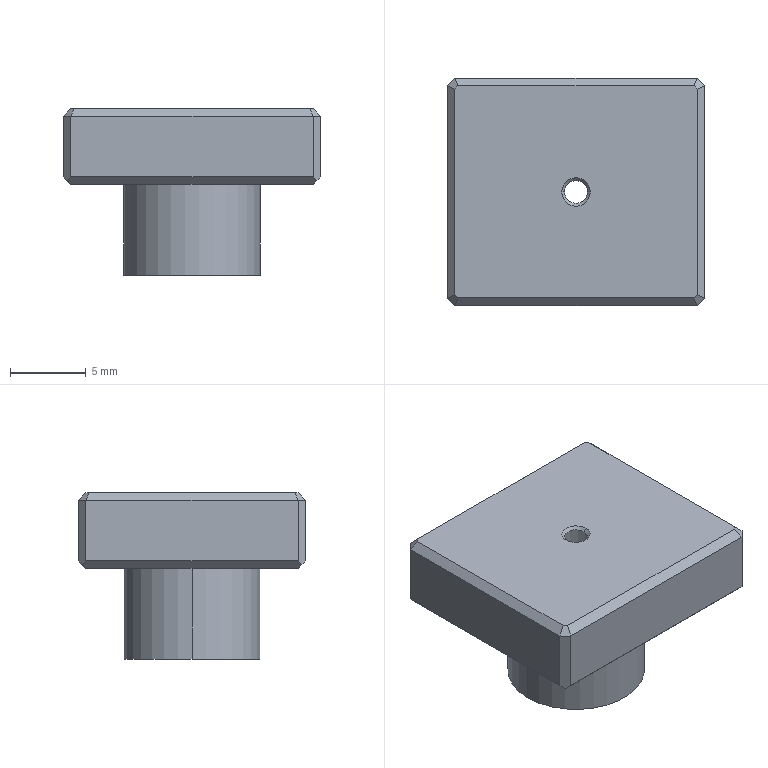Part | SolidWorks | features Chamfer 2, Extrusion 1, HoleWzd 1, ICE 1 | 1 solid | 31 faces | box 17 x 15 x 11 mm | volume 1494 mm3 | plane 23 | cone 4 | cylinder 4 | commonest cylinder face diameters 4.2 x2 9 x2
STEP:
#1=CARTESIAN_POINT('',(-0.7481,0.,10.812));
#2=VERTEX_POINT('',#1);
#3=CARTESIAN_POINT('',(0.7481,0.,10.812));
#4=VERTEX_POINT('',#3);
#5=CARTESIAN_POINT('',(0.,0.,10.812));
#6=DIRECTION('',(0.,0.,1.));
#7=DIRECTION('',(-1.,0.,0.));
#8=AXIS2_PLACEMENT_3D('',#5,#6,#7);
#9=CIRCLE('',#8,0.7481);
#10=EDGE_CURVE('',#2,#4,#9,.T.);
#11=ORIENTED_EDGE('',*,*,#10,.F.);
#12=CARTESIAN_POINT('',(-0.9357,0.,11.));
#13=VERTEX_POINT('',#12);
#14=CARTESIAN_POINT('',(-0.7481,0.,10.812));
#15=DIRECTION('',(-0.7071,0.,0.7071));
#16=VECTOR('',#15,1000.);
#17=LINE('',#14,#16);
#18=EDGE_CURVE('',#2,#13,#17,.T.);
#19=ORIENTED_EDGE('',*,*,#18,.T.);
#20=CARTESIAN_POINT('',(0.9357,0.,11.));
#21=VERTEX_POINT('',#20);
#22=CARTESIAN_POINT('',(0.,0.,11.));
#23=DIRECTION('',(0.,0.,-1.));
#24=DIRECTION('',(1.,0.,0.));
#25=AXIS2_PLACEMENT_3D('',#22,#23,#24);
#26=CIRCLE('',#25,0.9357);
#27=EDGE_CURVE('',#21,#13,#26,.T.);
#28=ORIENTED_EDGE('',*,*,#27,.F.);
#29=CARTESIAN_POINT('',(0.7481,0.,10.812));
#30=DIRECTION('',(0.7071,0.,0.7071));
#31=VECTOR('',#30,1000.);
#32=LINE('',#29,#31);
#33=EDGE_CURVE('',#4,#21,#32,.T.);
#34=ORIENTED_EDGE('',*,*,#33,.F.);
#35=EDGE_LOOP('',(#11,#19,#28,#34));
#36=FACE_OUTER_BOUND('',#35,.T.);
#37=CARTESIAN_POINT('',(0.,0.,10.812));
#38=DIRECTION('',(0.,0.,1.));
#39=DIRECTION('',(1.,0.,0.));
#40=AXIS2_PLACEMENT_3D('',#37,#38,#39);
#41=CONICAL_SURFACE('',#40,0.7481,0.7854);
#42=ADVANCED_FACE('',(#36),#41,.F.);
#43=CARTESIAN_POINT('',(2.1,0.,10.));
#44=VERTEX_POINT('',#43);
#45=CARTESIAN_POINT('',(-2.1,0.,10.));
#46=VERTEX_POINT('',#45);
#47=CARTESIAN_POINT('',(0.,0.,10.));
#48=DIRECTION('',(0.,0.,-1.));
#49=DIRECTION('',(-1.,0.,0.));
#50=AXIS2_PLACEMENT_3D('',#47,#48,#49);
#51=CIRCLE('',#50,2.1);
#52=EDGE_CURVE('',#44,#46,#51,.T.);
#53=ORIENTED_EDGE('',*,*,#52,.F.);
#54=CARTESIAN_POINT('',(2.1,0.,0.));
#55=VERTEX_POINT('',#54);
#56=CARTESIAN_POINT('',(2.1,0.,0.));
#57=DIRECTION('',(0.,0.,-1.));
#58=VECTOR('',#57,1000.);
#59=LINE('',#56,#58);
#60=EDGE_CURVE('',#44,#55,#59,.T.);
#61=ORIENTED_EDGE('',*,*,#60,.T.);
#62=CARTESIAN_POINT('',(-2.1,0.,0.));
#63=VERTEX_POINT('',#62);
#64=CARTESIAN_POINT('',(0.,0.,0.));
#65=DIRECTION('',(0.,0.,-1.));
#66=DIRECTION('',(-1.,0.,0.));
#67=AXIS2_PLACEMENT_3D('',#64,#65,#66);
#68=CIRCLE('',#67,2.1);
#69=EDGE_CURVE('',#55,#63,#68,.T.);
#70=ORIENTED_EDGE('',*,*,#69,.T.);
#71=CARTESIAN_POINT('',(-2.1,0.,0.));
#72=DIRECTION('',(0.,0.,-1.));
#73=VECTOR('',#72,1000.);
#74=LINE('',#71,#73);
#75=EDGE_CURVE('',#46,#63,#74,.T.);
#76=ORIENTED_EDGE('',*,*,#75,.F.);
#77=EDGE_LOOP('',(#53,#61,#70,#76));
#78=FACE_OUTER_BOUND('',#77,.T.);
#79=CARTESIAN_POINT('',(0.,0.,0.));
#80=DIRECTION('',(0.,0.,-1.));
#81=DIRECTION('',(-1.,0.,0.));
#82=AXIS2_PLACEMENT_3D('',#79,#80,#81);
#83=CYLINDRICAL_SURFACE('',#82,2.1);
#84=ADVANCED_FACE('',(#78),#83,.F.);
#85=ORIENTED_EDGE('',*,*,#10,.T.);
#86=CARTESIAN_POINT('',(2.1,0.,10.));
#87=DIRECTION('',(0.8572,0.,-0.515));
#88=VECTOR('',#87,1000.);
#89=LINE('',#86,#88);
#90=EDGE_CURVE('',#4,#44,#89,.T.);
#91=ORIENTED_EDGE('',*,*,#90,.T.);
#92=ORIENTED_EDGE('',*,*,#52,.T.);
#93=CARTESIAN_POINT('',(-2.1,0.,10.));
#94=DIRECTION('',(-0.8572,0.,-0.515));
#95=VECTOR('',#94,1000.);
#96=LINE('',#93,#95);
#97=EDGE_CURVE('',#2,#46,#96,.T.);
#98=ORIENTED_EDGE('',*,*,#97,.F.);
#99=EDGE_LOOP('',(#85,#91,#92,#98));
#100=FACE_OUTER_BOUND('',#99,.T.);
#101=CARTESIAN_POINT('',(0.,0.,10.));
#102=DIRECTION('',(0.,0.,-1.));
#103=DIRECTION('',(-1.,0.,0.));
#104=AXIS2_PLACEMENT_3D('',#101,#102,#103);
#105=CONICAL_SURFACE('',#104,2.1,1.03);
#106=ADVANCED_FACE('',(#100),#105,.F.);
#107=CARTESIAN_POINT('',(4.5,0.,6.));
#108=VERTEX_POINT('',#107);
#109=CARTESIAN_POINT('',(-4.5,0.,6.));
#110=VERTEX_POINT('',#109);
#111=CARTESIAN_POINT('',(0.,0.,6.));
#112=DIRECTION('',(0.,0.,1.));
#113=DIRECTION('',(1.,0.,0.));
#114=AXIS2_PLACEMENT_3D('',#111,#112,#113);
#115=CIRCLE('',#114,4.5);
#116=EDGE_CURVE('',#108,#110,#115,.T.);
#117=ORIENTED_EDGE('',*,*,#116,.F.);
#118=CARTESIAN_POINT('',(4.5,0.,0.));
#119=VERTEX_POINT('',#118);
#120=CARTESIAN_POINT('',(4.5,0.,6.));
#121=DIRECTION('',(0.,0.,-1.));
#122=VECTOR('',#121,1000.);
#123=LINE('',#120,#122);
#124=EDGE_CURVE('',#108,#119,#123,.T.);
#125=ORIENTED_EDGE('',*,*,#124,.T.);
#126=CARTESIAN_POINT('',(-4.5,0.,0.));
#127=VERTEX_POINT('',#126);
#128=CARTESIAN_POINT('',(0.,0.,0.));
#129=DIRECTION('',(0.,0.,1.));
#130=DIRECTION('',(1.,0.,0.));
#131=AXIS2_PLACEMENT_3D('',#128,#129,#130);
#132=CIRCLE('',#131,4.5);
#133=EDGE_CURVE('',#119,#127,#132,.T.);
#134=ORIENTED_EDGE('',*,*,#133,.T.);
#135=CARTESIAN_POINT('',(-4.5,0.,6.));
#136=DIRECTION('',(0.,0.,-1.));
#137=VECTOR('',#136,1000.);
#138=LINE('',#135,#137);
#139=EDGE_CURVE('',#110,#127,#138,.T.);
#140=ORIENTED_EDGE('',*,*,#139,.F.);
#141=EDGE_LOOP('',(#117,#125,#134,#140));
#142=FACE_OUTER_BOUND('',#141,.T.);
#143=CARTESIAN_POINT('',(0.,0.,6.));
#144=DIRECTION('',(0.,0.,-1.));
#145=DIRECTION('',(-1.,0.,0.));
#146=AXIS2_PLACEMENT_3D('',#143,#144,#145);
#147=CYLINDRICAL_SURFACE('',#146,4.5);
#148=ADVANCED_FACE('',(#142),#147,.T.);
#149=ORIENTED_EDGE('',*,*,#124,.F.);
#150=CARTESIAN_POINT('',(0.,0.,6.));
#151=DIRECTION('',(0.,0.,1.));
#152=DIRECTION('',(1.,0.,0.));
#153=AXIS2_PLACEMENT_3D('',#150,#151,#152);
#154=CIRCLE('',#153,4.5);
#155=EDGE_CURVE('',#110,#108,#154,.T.);
#156=ORIENTED_EDGE('',*,*,#155,.F.);
#157=ORIENTED_EDGE('',*,*,#139,.T.);
#158=CARTESIAN_POINT('',(0.,0.,0.));
#159=DIRECTION('',(0.,0.,1.));
#160=DIRECTION('',(1.,0.,0.));
#161=AXIS2_PLACEMENT_3D('',#158,#159,#160);
#162=CIRCLE('',#161,4.5);
#163=EDGE_CURVE('',#127,#119,#162,.T.);
#164=ORIENTED_EDGE('',*,*,#163,.T.);
#165=EDGE_LOOP('',(#149,#156,#157,#164));
#166=FACE_OUTER_BOUND('',#165,.T.);
#167=CARTESIAN_POINT('',(0.,0.,6.));
#168=DIRECTION('',(0.,0.,-1.));
#169=DIRECTION('',(-1.,0.,0.));
#170=AXIS2_PLACEMENT_3D('',#167,#168,#169);
#171=CYLINDRICAL_SURFACE('',#170,4.5);
#172=ADVANCED_FACE('',(#166),#171,.T.);
#173=CARTESIAN_POINT('',(0.,0.,0.));
#174=DIRECTION('',(0.,0.,-1.));
#175=DIRECTION('',(-1.,0.,0.));
#176=AXIS2_PLACEMENT_3D('',#173,#174,#175);
#177=CIRCLE('',#176,2.1);
#178=EDGE_CURVE('',#63,#55,#177,.T.);
#179=ORIENTED_EDGE('',*,*,#178,.F.);
#180=ORIENTED_EDGE('',*,*,#69,.F.);
#181=EDGE_LOOP('',(#179,#180));
#182=FACE_BOUND('',#181,.T.);
#183=ORIENTED_EDGE('',*,*,#163,.F.);
#184=ORIENTED_EDGE('',*,*,#133,.F.);
#185=EDGE_LOOP('',(#183,#184));
#186=FACE_OUTER_BOUND('',#185,.T.);
#187=CARTESIAN_POINT('',(0.,0.,0.));
#188=DIRECTION('',(0.,0.,1.));
#189=DIRECTION('',(1.,0.,0.));
#190=AXIS2_PLACEMENT_3D('',#187,#188,#189);
#191=PLANE('',#190);
#192=ADVANCED_FACE('',(#182,#186),#191,.F.);
#193=CARTESIAN_POINT('',(8.5,7.,6.5));
#194=VERTEX_POINT('',#193);
#195=CARTESIAN_POINT('',(8.5,7.,10.5));
#196=VERTEX_POINT('',#195);
#197=CARTESIAN_POINT('',(8.5,7.,11.));
#198=DIRECTION('',(0.,0.,1.));
#199=VECTOR('',#198,1000.);
#200=LINE('',#197,#199);
#201=EDGE_CURVE('',#194,#196,#200,.T.);
#202=ORIENTED_EDGE('',*,*,#201,.T.);
#203=CARTESIAN_POINT('',(8.5,-7.,10.5));
#204=VERTEX_POINT('',#203);
#205=CARTESIAN_POINT('',(8.5,-7.,10.5));
#206=DIRECTION('',(0.,-1.,0.));
#207=VECTOR('',#206,1000.);
#208=LINE('',#205,#207);
#209=EDGE_CURVE('',#196,#204,#208,.T.);
#210=ORIENTED_EDGE('',*,*,#209,.T.);
#211=CARTESIAN_POINT('',(8.5,-7.,6.5));
#212=VERTEX_POINT('',#211);
#213=CARTESIAN_POINT('',(8.5,-7.,11.));
#214=DIRECTION('',(0.,0.,-1.));
#215=VECTOR('',#214,1000.);
#216=LINE('',#213,#215);
#217=EDGE_CURVE('',#204,#212,#216,.T.);
#218=ORIENTED_EDGE('',*,*,#217,.T.);
#219=CARTESIAN_POINT('',(8.5,7.5,6.5));
#220=DIRECTION('',(0.,1.,0.));
#221=VECTOR('',#220,1000.);
#222=LINE('',#219,#221);
#223=EDGE_CURVE('',#212,#194,#222,.T.);
#224=ORIENTED_EDGE('',*,*,#223,.T.);
#225=EDGE_LOOP('',(#202,#210,#218,#224));
#226=FACE_OUTER_BOUND('',#225,.T.);
#227=CARTESIAN_POINT('',(8.5,7.5,11.));
#228=DIRECTION('',(-1.,0.,0.));
#229=DIRECTION('',(0.,-1.,0.));
#230=AXIS2_PLACEMENT_3D('',#227,#228,#229);
#231=PLANE('',#230);
#232=ADVANCED_FACE('',(#226),#231,.F.);
#233=CARTESIAN_POINT('',(-8.,7.5,6.5));
#234=VERTEX_POINT('',#233);
#235=CARTESIAN_POINT('',(-8.,7.5,10.5));
#236=VERTEX_POINT('',#235);
#237=CARTESIAN_POINT('',(-8.,7.5,11.));
#238=DIRECTION('',(0.,0.,1.));
#239=VECTOR('',#238,1000.);
#240=LINE('',#237,#239);
#241=EDGE_CURVE('',#234,#236,#240,.T.);
#242=ORIENTED_EDGE('',*,*,#241,.T.);
#243=CARTESIAN_POINT('',(8.,7.5,10.5));
#244=VERTEX_POINT('',#243);
#245=CARTESIAN_POINT('',(8.,7.5,10.5));
#246=DIRECTION('',(1.,0.,0.));
#247=VECTOR('',#246,1000.);
#248=LINE('',#245,#247);
#249=EDGE_CURVE('',#236,#244,#248,.T.);
#250=ORIENTED_EDGE('',*,*,#249,.T.);
#251=CARTESIAN_POINT('',(8.,7.5,6.5));
#252=VERTEX_POINT('',#251);
#253=CARTESIAN_POINT('',(8.,7.5,11.));
#254=DIRECTION('',(0.,0.,-1.));
#255=VECTOR('',#254,1000.);
#256=LINE('',#253,#255);
#257=EDGE_CURVE('',#244,#252,#256,.T.);
#258=ORIENTED_EDGE('',*,*,#257,.T.);
#259=CARTESIAN_POINT('',(-8.5,7.5,6.5));
#260=DIRECTION('',(-1.,0.,0.));
#261=VECTOR('',#260,1000.);
#262=LINE('',#259,#261);
#263=EDGE_CURVE('',#252,#234,#262,.T.);
#264=ORIENTED_EDGE('',*,*,#263,.T.);
#265=EDGE_LOOP('',(#242,#250,#258,#264));
#266=FACE_OUTER_BOUND('',#265,.T.);
#267=CARTESIAN_POINT('',(-8.5,7.5,11.));
#268=DIRECTION('',(0.,-1.,0.));
#269=DIRECTION('',(0.,0.,-1.));
#270=AXIS2_PLACEMENT_3D('',#267,#268,#269);
#271=PLANE('',#270);
#272=ADVANCED_FACE('',(#266),#271,.F.);
#273=CARTESIAN_POINT('',(-8.5,-7.,6.5));
#274=VERTEX_POINT('',#273);
#275=CARTESIAN_POINT('',(-8.5,-7.,10.5));
#276=VERTEX_POINT('',#275);
#277=CARTESIAN_POINT('',(-8.5,-7.,11.));
#278=DIRECTION('',(0.,0.,1.));
#279=VECTOR('',#278,1000.);
#280=LINE('',#277,#279);
#281=EDGE_CURVE('',#274,#276,#280,.T.);
#282=ORIENTED_EDGE('',*,*,#281,.T.);
#283=CARTESIAN_POINT('',(-8.5,7.,10.5));
#284=VERTEX_POINT('',#283);
#285=CARTESIAN_POINT('',(-8.5,7.,10.5));
#286=DIRECTION('',(0.,1.,0.));
#287=VECTOR('',#286,1000.);
#288=LINE('',#285,#287);
#289=EDGE_CURVE('',#276,#284,#288,.T.);
#290=ORIENTED_EDGE('',*,*,#289,.T.);
#291=CARTESIAN_POINT('',(-8.5,7.,6.5));
#292=VERTEX_POINT('',#291);
#293=CARTESIAN_POINT('',(-8.5,7.,11.));
#294=DIRECTION('',(0.,0.,-1.));
#295=VECTOR('',#294,1000.);
#296=LINE('',#293,#295);
#297=EDGE_CURVE('',#284,#292,#296,.T.);
#298=ORIENTED_EDGE('',*,*,#297,.T.);
#299=CARTESIAN_POINT('',(-8.5,7.5,6.5));
#300=DIRECTION('',(0.,-1.,0.));
#301=VECTOR('',#300,1000.);
#302=LINE('',#299,#301);
#303=EDGE_CURVE('',#292,#274,#302,.T.);
#304=ORIENTED_EDGE('',*,*,#303,.T.);
#305=EDGE_LOOP('',(#282,#290,#298,#304));
#306=FACE_OUTER_BOUND('',#305,.T.);
#307=CARTESIAN_POINT('',(-8.5,7.5,11.));
#308=DIRECTION('',(1.,0.,0.));
#309=DIRECTION('',(0.,1.,0.));
#310=AXIS2_PLACEMENT_3D('',#307,#308,#309);
#311=PLANE('',#310);
#312=ADVANCED_FACE('',(#306),#311,.F.);
#313=CARTESIAN_POINT('',(8.,-7.5,6.5));
#314=VERTEX_POINT('',#313);
#315=CARTESIAN_POINT('',(8.,-7.5,10.5));
#316=VERTEX_POINT('',#315);
#317=CARTESIAN_POINT('',(8.,-7.5,11.));
#318=DIRECTION('',(0.,0.,1.));
#319=VECTOR('',#318,1000.);
#320=LINE('',#317,#319);
#321=EDGE_CURVE('',#314,#316,#320,.T.);
#322=ORIENTED_EDGE('',*,*,#321,.T.);
#323=CARTESIAN_POINT('',(-8.,-7.5,10.5));
#324=VERTEX_POINT('',#323);
#325=CARTESIAN_POINT('',(-8.,-7.5,10.5));
#326=DIRECTION('',(-1.,0.,0.));
#327=VECTOR('',#326,1000.);
#328=LINE('',#325,#327);
#329=EDGE_CURVE('',#316,#324,#328,.T.);
#330=ORIENTED_EDGE('',*,*,#329,.T.);
#331=CARTESIAN_POINT('',(-8.,-7.5,6.5));
#332=VERTEX_POINT('',#331);
#333=CARTESIAN_POINT('',(-8.,-7.5,11.));
#334=DIRECTION('',(0.,0.,-1.));
#335=VECTOR('',#334,1000.);
#336=LINE('',#333,#335);
#337=EDGE_CURVE('',#324,#332,#336,.T.);
#338=ORIENTED_EDGE('',*,*,#337,.T.);
#339=CARTESIAN_POINT('',(-8.5,-7.5,6.5));
#340=DIRECTION('',(1.,0.,0.));
#341=VECTOR('',#340,1000.);
#342=LINE('',#339,#341);
#343=EDGE_CURVE('',#332,#314,#342,.T.);
#344=ORIENTED_EDGE('',*,*,#343,.T.);
#345=EDGE_LOOP('',(#322,#330,#338,#344));
#346=FACE_OUTER_BOUND('',#345,.T.);
#347=CARTESIAN_POINT('',(-8.5,-7.5,11.));
#348=DIRECTION('',(0.,1.,0.));
#349=DIRECTION('',(0.,0.,1.));
#350=AXIS2_PLACEMENT_3D('',#347,#348,#349);
#351=PLANE('',#350);
#352=ADVANCED_FACE('',(#346),#351,.F.);
#353=CARTESIAN_POINT('',(-8.,6.793,11.));
#354=VERTEX_POINT('',#353);
#355=CARTESIAN_POINT('',(-8.,-6.793,11.));
#356=VERTEX_POINT('',#355);
#357=CARTESIAN_POINT('',(-8.,-7.,11.));
#358=DIRECTION('',(0.,-1.,0.));
#359=VECTOR('',#358,1000.);
#360=LINE('',#357,#359);
#361=EDGE_CURVE('',#354,#356,#360,.T.);
#362=ORIENTED_EDGE('',*,*,#361,.T.);
#363=CARTESIAN_POINT('',(-7.793,-7.,11.));
#364=VERTEX_POINT('',#363);
#365=CARTESIAN_POINT('',(-7.396,-7.396,11.));
#366=DIRECTION('',(0.7071,-0.7071,0.));
#367=VECTOR('',#366,1000.);
#368=LINE('',#365,#367);
#369=EDGE_CURVE('',#356,#364,#368,.T.);
#370=ORIENTED_EDGE('',*,*,#369,.T.);
#371=CARTESIAN_POINT('',(7.793,-7.,11.));
#372=VERTEX_POINT('',#371);
#373=CARTESIAN_POINT('',(8.,-7.,11.));
#374=DIRECTION('',(1.,0.,0.));
#375=VECTOR('',#374,1000.);
#376=LINE('',#373,#375);
#377=EDGE_CURVE('',#364,#372,#376,.T.);
#378=ORIENTED_EDGE('',*,*,#377,.T.);
#379=CARTESIAN_POINT('',(8.,-6.793,11.));
#380=VERTEX_POINT('',#379);
#381=CARTESIAN_POINT('',(7.396,-7.396,11.));
#382=DIRECTION('',(0.7071,0.7071,0.));
#383=VECTOR('',#382,1000.);
#384=LINE('',#381,#383);
#385=EDGE_CURVE('',#372,#380,#384,.T.);
#386=ORIENTED_EDGE('',*,*,#385,.T.);
#387=CARTESIAN_POINT('',(8.,6.793,11.));
#388=VERTEX_POINT('',#387);
#389=CARTESIAN_POINT('',(8.,7.,11.));
#390=DIRECTION('',(0.,1.,0.));
#391=VECTOR('',#390,1000.);
#392=LINE('',#389,#391);
#393=EDGE_CURVE('',#380,#388,#392,.T.);
#394=ORIENTED_EDGE('',*,*,#393,.T.);
#395=CARTESIAN_POINT('',(7.793,7.,11.));
#396=VERTEX_POINT('',#395);
#397=CARTESIAN_POINT('',(7.396,7.396,11.));
#398=DIRECTION('',(-0.7071,0.7071,0.));
#399=VECTOR('',#398,1000.);
#400=LINE('',#397,#399);
#401=EDGE_CURVE('',#388,#396,#400,.T.);
#402=ORIENTED_EDGE('',*,*,#401,.T.);
#403=CARTESIAN_POINT('',(-7.793,7.,11.));
#404=VERTEX_POINT('',#403);
#405=CARTESIAN_POINT('',(-8.,7.,11.));
#406=DIRECTION('',(-1.,0.,0.));
#407=VECTOR('',#406,1000.);
#408=LINE('',#405,#407);
#409=EDGE_CURVE('',#396,#404,#408,.T.);
#410=ORIENTED_EDGE('',*,*,#409,.T.);
#411=CARTESIAN_POINT('',(-7.396,7.396,11.));
#412=DIRECTION('',(-0.7071,-0.7071,0.));
#413=VECTOR('',#412,1000.);
#414=LINE('',#411,#413);
#415=EDGE_CURVE('',#404,#354,#414,.T.);
#416=ORIENTED_EDGE('',*,*,#415,.T.);
#417=EDGE_LOOP('',(#362,#370,#378,#386,#394,#402,#410,#416));
#418=FACE_OUTER_BOUND('',#417,.T.);
#419=ORIENTED_EDGE('',*,*,#27,.T.);
#420=CARTESIAN_POINT('',(0.,0.,11.));
#421=DIRECTION('',(0.,0.,-1.));
#422=DIRECTION('',(1.,0.,0.));
#423=AXIS2_PLACEMENT_3D('',#420,#421,#422);
#424=CIRCLE('',#423,0.9357);
#425=EDGE_CURVE('',#13,#21,#424,.T.);
#426=ORIENTED_EDGE('',*,*,#425,.T.);
#427=EDGE_LOOP('',(#419,#426));
#428=FACE_BOUND('',#427,.T.);
#429=CARTESIAN_POINT('',(0.,0.,11.));
#430=DIRECTION('',(0.,0.,1.));
#431=DIRECTION('',(1.,0.,0.));
#432=AXIS2_PLACEMENT_3D('',#429,#430,#431);
#433=PLANE('',#432);
#434=ADVANCED_FACE('',(#418,#428),#433,.T.);
#435=CARTESIAN_POINT('',(-8.,-7.,6.));
#436=VERTEX_POINT('',#435);
#437=CARTESIAN_POINT('',(-8.,7.,6.));
#438=VERTEX_POINT('',#437);
#439=CARTESIAN_POINT('',(-8.,0.,6.));
#440=DIRECTION('',(0.,1.,0.));
#441=VECTOR('',#440,1000.);
#442=LINE('',#439,#441);
#443=EDGE_CURVE('',#436,#438,#442,.T.);
#444=ORIENTED_EDGE('',*,*,#443,.T.);
#445=CARTESIAN_POINT('',(8.,7.,6.));
#446=VERTEX_POINT('',#445);
#447=CARTESIAN_POINT('',(0.,7.,6.));
#448=DIRECTION('',(1.,0.,0.));
#449=VECTOR('',#448,1000.);
#450=LINE('',#447,#449);
#451=EDGE_CURVE('',#438,#446,#450,.T.);
#452=ORIENTED_EDGE('',*,*,#451,.T.);
#453=CARTESIAN_POINT('',(8.,-7.,6.));
#454=VERTEX_POINT('',#453);
#455=CARTESIAN_POINT('',(8.,0.,6.));
#456=DIRECTION('',(0.,-1.,0.));
#457=VECTOR('',#456,1000.);
#458=LINE('',#455,#457);
#459=EDGE_CURVE('',#446,#454,#458,.T.);
#460=ORIENTED_EDGE('',*,*,#459,.T.);
#461=CARTESIAN_POINT('',(0.,-7.,6.));
#462=DIRECTION('',(-1.,0.,0.));
#463=VECTOR('',#462,1000.);
#464=LINE('',#461,#463);
#465=EDGE_CURVE('',#454,#436,#464,.T.);
#466=ORIENTED_EDGE('',*,*,#465,.T.);
#467=EDGE_LOOP('',(#444,#452,#460,#466));
#468=FACE_OUTER_BOUND('',#467,.T.);
#469=ORIENTED_EDGE('',*,*,#155,.T.);
#470=ORIENTED_EDGE('',*,*,#116,.T.);
#471=EDGE_LOOP('',(#469,#470));
#472=FACE_BOUND('',#471,.T.);
#473=CARTESIAN_POINT('',(0.,0.,6.));
#474=DIRECTION('',(0.,0.,1.));
#475=DIRECTION('',(1.,0.,0.));
#476=AXIS2_PLACEMENT_3D('',#473,#474,#475);
#477=PLANE('',#476);
#478=ADVANCED_FACE('',(#468,#472),#477,.F.);
#479=ORIENTED_EDGE('',*,*,#90,.F.);
#480=CARTESIAN_POINT('',(0.,0.,10.812));
#481=DIRECTION('',(0.,0.,1.));
#482=DIRECTION('',(-1.,0.,0.));
#483=AXIS2_PLACEMENT_3D('',#480,#481,#482);
#484=CIRCLE('',#483,0.7481);
#485=EDGE_CURVE('',#4,#2,#484,.T.);
#486=ORIENTED_EDGE('',*,*,#485,.T.);
#487=ORIENTED_EDGE('',*,*,#97,.T.);
#488=CARTESIAN_POINT('',(0.,0.,10.));
#489=DIRECTION('',(0.,0.,-1.));
#490=DIRECTION('',(-1.,0.,0.));
#491=AXIS2_PLACEMENT_3D('',#488,#489,#490);
#492=CIRCLE('',#491,2.1);
#493=EDGE_CURVE('',#46,#44,#492,.T.);
#494=ORIENTED_EDGE('',*,*,#493,.T.);
#495=EDGE_LOOP('',(#479,#486,#487,#494));
#496=FACE_OUTER_BOUND('',#495,.T.);
#497=CARTESIAN_POINT('',(0.,0.,10.));
#498=DIRECTION('',(0.,0.,-1.));
#499=DIRECTION('',(-1.,0.,0.));
#500=AXIS2_PLACEMENT_3D('',#497,#498,#499);
#501=CONICAL_SURFACE('',#500,2.1,1.03);
#502=ADVANCED_FACE('',(#496),#501,.F.);
#503=ORIENTED_EDGE('',*,*,#60,.F.);
#504=ORIENTED_EDGE('',*,*,#493,.F.);
#505=ORIENTED_EDGE('',*,*,#75,.T.);
#506=ORIENTED_EDGE('',*,*,#178,.T.);
#507=EDGE_LOOP('',(#503,#504,#505,#506));
#508=FACE_OUTER_BOUND('',#507,.T.);
#509=CARTESIAN_POINT('',(0.,0.,0.));
#510=DIRECTION('',(0.,0.,-1.));
#511=DIRECTION('',(-1.,0.,0.));
#512=AXIS2_PLACEMENT_3D('',#509,#510,#511);
#513=CYLINDRICAL_SURFACE('',#512,2.1);
#514=ADVANCED_FACE('',(#508),#513,.F.);
#515=ORIENTED_EDGE('',*,*,#217,.F.);
#516=CARTESIAN_POINT('',(8.5,-7.,10.5));
#517=DIRECTION('',(-0.7071,-0.7071,0.));
#518=VECTOR('',#517,1000.);
#519=LINE('',#516,#518);
#520=EDGE_CURVE('',#204,#316,#519,.T.);
#521=ORIENTED_EDGE('',*,*,#520,.T.);
#522=ORIENTED_EDGE('',*,*,#321,.F.);
#523=CARTESIAN_POINT('',(8.25,-7.25,6.25));
#524=VERTEX_POINT('',#523);
#525=CARTESIAN_POINT('',(6.833,-8.667,7.667));
#526=DIRECTION('',(0.5774,0.5774,-0.5774));
#527=VECTOR('',#526,1000.);
#528=LINE('',#525,#527);
#529=EDGE_CURVE('',#314,#524,#528,.T.);
#530=ORIENTED_EDGE('',*,*,#529,.T.);
#531=CARTESIAN_POINT('',(10.,-5.5,8.));
#532=DIRECTION('',(0.5774,0.5774,0.5774));
#533=VECTOR('',#532,1000.);
#534=LINE('',#531,#533);
#535=EDGE_CURVE('',#524,#212,#534,.T.);
#536=ORIENTED_EDGE('',*,*,#535,.T.);
#537=EDGE_LOOP('',(#515,#521,#522,#530,#536));
#538=FACE_OUTER_BOUND('',#537,.T.);
#539=CARTESIAN_POINT('',(8.5,-7.,11.));
#540=DIRECTION('',(-0.7071,0.7071,0.));
#541=DIRECTION('',(0.,0.,-1.));
#542=AXIS2_PLACEMENT_3D('',#539,#540,#541);
#543=PLANE('',#542);
#544=ADVANCED_FACE('',(#538),#543,.F.);
#545=ORIENTED_EDGE('',*,*,#257,.F.);
#546=CARTESIAN_POINT('',(8.,7.5,10.5));
#547=DIRECTION('',(0.7071,-0.7071,0.));
#548=VECTOR('',#547,1000.);
#549=LINE('',#546,#548);
#550=EDGE_CURVE('',#244,#196,#549,.T.);
#551=ORIENTED_EDGE('',*,*,#550,.T.);
#552=ORIENTED_EDGE('',*,*,#201,.F.);
#553=CARTESIAN_POINT('',(8.25,7.25,6.25));
#554=VERTEX_POINT('',#553);
#555=CARTESIAN_POINT('',(9.667,5.833,7.667));
#556=DIRECTION('',(-0.5774,0.5774,-0.5774));
#557=VECTOR('',#556,1000.);
#558=LINE('',#555,#557);
#559=EDGE_CURVE('',#194,#554,#558,.T.);
#560=ORIENTED_EDGE('',*,*,#559,.T.);
#561=CARTESIAN_POINT('',(6.5,9.,8.));
#562=DIRECTION('',(-0.5774,0.5774,0.5774));
#563=VECTOR('',#562,1000.);
#564=LINE('',#561,#563);
#565=EDGE_CURVE('',#554,#252,#564,.T.);
#566=ORIENTED_EDGE('',*,*,#565,.T.);
#567=EDGE_LOOP('',(#545,#551,#552,#560,#566));
#568=FACE_OUTER_BOUND('',#567,.T.);
#569=CARTESIAN_POINT('',(8.,7.5,11.));
#570=DIRECTION('',(-0.7071,-0.7071,0.));
#571=DIRECTION('',(0.,0.,-1.));
#572=AXIS2_PLACEMENT_3D('',#569,#570,#571);
#573=PLANE('',#572);
#574=ADVANCED_FACE('',(#568),#573,.F.);
#575=ORIENTED_EDGE('',*,*,#337,.F.);
#576=CARTESIAN_POINT('',(-8.,-7.5,10.5));
#577=DIRECTION('',(-0.7071,0.7071,0.));
#578=VECTOR('',#577,1000.);
#579=LINE('',#576,#578);
#580=EDGE_CURVE('',#324,#276,#579,.T.);
#581=ORIENTED_EDGE('',*,*,#580,.T.);
#582=ORIENTED_EDGE('',*,*,#281,.F.);
#583=CARTESIAN_POINT('',(-8.25,-7.25,6.25));
#584=VERTEX_POINT('',#583);
#585=CARTESIAN_POINT('',(-9.667,-5.833,7.667));
#586=DIRECTION('',(0.5774,-0.5774,-0.5774));
#587=VECTOR('',#586,1000.);
#588=LINE('',#585,#587);
#589=EDGE_CURVE('',#274,#584,#588,.T.);
#590=ORIENTED_EDGE('',*,*,#589,.T.);
#591=CARTESIAN_POINT('',(-6.5,-9.,8.));
#592=DIRECTION('',(0.5774,-0.5774,0.5774));
#593=VECTOR('',#592,1000.);
#594=LINE('',#591,#593);
#595=EDGE_CURVE('',#584,#332,#594,.T.);
#596=ORIENTED_EDGE('',*,*,#595,.T.);
#597=EDGE_LOOP('',(#575,#581,#582,#590,#596));
#598=FACE_OUTER_BOUND('',#597,.T.);
#599=CARTESIAN_POINT('',(-8.,-7.5,11.));
#600=DIRECTION('',(0.7071,0.7071,0.));
#601=DIRECTION('',(0.,0.,-1.));
#602=AXIS2_PLACEMENT_3D('',#599,#600,#601);
#603=PLANE('',#602);
#604=ADVANCED_FACE('',(#598),#603,.F.);
#605=ORIENTED_EDGE('',*,*,#297,.F.);
#606=CARTESIAN_POINT('',(-8.5,7.,10.5));
#607=DIRECTION('',(0.7071,0.7071,0.));
#608=VECTOR('',#607,1000.);
#609=LINE('',#606,#608);
#610=EDGE_CURVE('',#284,#236,#609,.T.);
#611=ORIENTED_EDGE('',*,*,#610,.T.);
#612=ORIENTED_EDGE('',*,*,#241,.F.);
#613=CARTESIAN_POINT('',(-8.25,7.25,6.25));
#614=VERTEX_POINT('',#613);
#615=CARTESIAN_POINT('',(-6.833,8.667,7.667));
#616=DIRECTION('',(-0.5774,-0.5774,-0.5774));
#617=VECTOR('',#616,1000.);
#618=LINE('',#615,#617);
#619=EDGE_CURVE('',#234,#614,#618,.T.);
#620=ORIENTED_EDGE('',*,*,#619,.T.);
#621=CARTESIAN_POINT('',(-10.,5.5,8.));
#622=DIRECTION('',(-0.5774,-0.5774,0.5774));
#623=VECTOR('',#622,1000.);
#624=LINE('',#621,#623);
#625=EDGE_CURVE('',#614,#292,#624,.T.);
#626=ORIENTED_EDGE('',*,*,#625,.T.);
#627=EDGE_LOOP('',(#605,#611,#612,#620,#626));
#628=FACE_OUTER_BOUND('',#627,.T.);
#629=CARTESIAN_POINT('',(-8.5,7.,11.));
#630=DIRECTION('',(0.7071,-0.7071,0.));
#631=DIRECTION('',(0.,0.,-1.));
#632=AXIS2_PLACEMENT_3D('',#629,#630,#631);
#633=PLANE('',#632);
#634=ADVANCED_FACE('',(#628),#633,.F.);
#635=CARTESIAN_POINT('',(6.704,6.256,12.296));
#636=DIRECTION('',(-0.6786,-0.2811,0.6786));
#637=VECTOR('',#636,1000.);
#638=LINE('',#635,#637);
#639=EDGE_CURVE('',#196,#388,#638,.T.);
#640=ORIENTED_EDGE('',*,*,#639,.F.);
#641=ORIENTED_EDGE('',*,*,#550,.F.);
#642=CARTESIAN_POINT('',(7.837,7.107,10.893));
#643=DIRECTION('',(0.2811,0.6786,-0.6786));
#644=VECTOR('',#643,1000.);
#645=LINE('',#642,#644);
#646=EDGE_CURVE('',#396,#244,#645,.T.);
#647=ORIENTED_EDGE('',*,*,#646,.F.);
#648=ORIENTED_EDGE('',*,*,#401,.F.);
#649=EDGE_LOOP('',(#640,#641,#647,#648));
#650=FACE_OUTER_BOUND('',#649,.T.);
#651=CARTESIAN_POINT('',(7.396,7.396,11.));
#652=DIRECTION('',(0.5,0.5,0.7071));
#653=DIRECTION('',(0.7071,-0.7071,0.));
#654=AXIS2_PLACEMENT_3D('',#651,#652,#653);
#655=PLANE('',#654);
#656=ADVANCED_FACE('',(#650),#655,.T.);
#657=ORIENTED_EDGE('',*,*,#646,.T.);
#658=ORIENTED_EDGE('',*,*,#249,.F.);
#659=CARTESIAN_POINT('',(-7.177,5.514,12.486));
#660=DIRECTION('',(-0.2811,0.6786,-0.6786));
#661=VECTOR('',#660,1000.);
#662=LINE('',#659,#661);
#663=EDGE_CURVE('',#404,#236,#662,.T.);
#664=ORIENTED_EDGE('',*,*,#663,.F.);
#665=ORIENTED_EDGE('',*,*,#409,.F.);
#666=EDGE_LOOP('',(#657,#658,#664,#665));
#667=FACE_OUTER_BOUND('',#666,.T.);
#668=CARTESIAN_POINT('',(0.,7.,11.));
#669=DIRECTION('',(0.,0.7071,0.7071));
#670=DIRECTION('',(1.,0.,0.));
#671=AXIS2_PLACEMENT_3D('',#668,#669,#670);
#672=PLANE('',#671);
#673=ADVANCED_FACE('',(#667),#672,.T.);
#674=ORIENTED_EDGE('',*,*,#639,.T.);
#675=ORIENTED_EDGE('',*,*,#393,.F.);
#676=CARTESIAN_POINT('',(7.837,-6.725,11.163));
#677=DIRECTION('',(-0.6786,0.2811,0.6786));
#678=VECTOR('',#677,1000.);
#679=LINE('',#676,#678);
#680=EDGE_CURVE('',#204,#380,#679,.T.);
#681=ORIENTED_EDGE('',*,*,#680,.F.);
#682=ORIENTED_EDGE('',*,*,#209,.F.);
#683=EDGE_LOOP('',(#674,#675,#681,#682));
#684=FACE_OUTER_BOUND('',#683,.T.);
#685=CARTESIAN_POINT('',(8.,0.,11.));
#686=DIRECTION('',(0.7071,0.,0.7071));
#687=DIRECTION('',(0.,-1.,0.));
#688=AXIS2_PLACEMENT_3D('',#685,#686,#687);
#689=PLANE('',#688);
#690=ADVANCED_FACE('',(#684),#689,.T.);
#691=ORIENTED_EDGE('',*,*,#663,.T.);
#692=ORIENTED_EDGE('',*,*,#610,.F.);
#693=CARTESIAN_POINT('',(-7.837,6.725,11.163));
#694=DIRECTION('',(-0.6786,0.2811,-0.6786));
#695=VECTOR('',#694,1000.);
#696=LINE('',#693,#695);
#697=EDGE_CURVE('',#354,#284,#696,.T.);
#698=ORIENTED_EDGE('',*,*,#697,.F.);
#699=ORIENTED_EDGE('',*,*,#415,.F.);
#700=EDGE_LOOP('',(#691,#692,#698,#699));
#701=FACE_OUTER_BOUND('',#700,.T.);
#702=CARTESIAN_POINT('',(-7.396,7.396,11.));
#703=DIRECTION('',(-0.5,0.5,0.7071));
#704=DIRECTION('',(0.7071,0.7071,0.));
#705=AXIS2_PLACEMENT_3D('',#702,#703,#704);
#706=PLANE('',#705);
#707=ADVANCED_FACE('',(#701),#706,.T.);
#708=ORIENTED_EDGE('',*,*,#680,.T.);
#709=ORIENTED_EDGE('',*,*,#385,.F.);
#710=CARTESIAN_POINT('',(7.177,-5.514,12.486));
#711=DIRECTION('',(-0.2811,0.6786,0.6786));
#712=VECTOR('',#711,1000.);
#713=LINE('',#710,#712);
#714=EDGE_CURVE('',#316,#372,#713,.T.);
#715=ORIENTED_EDGE('',*,*,#714,.F.);
#716=ORIENTED_EDGE('',*,*,#520,.F.);
#717=EDGE_LOOP('',(#708,#709,#715,#716));
#718=FACE_OUTER_BOUND('',#717,.T.);
#719=CARTESIAN_POINT('',(7.396,-7.396,11.));
#720=DIRECTION('',(0.5,-0.5,0.7071));
#721=DIRECTION('',(-0.7071,-0.7071,0.));
#722=AXIS2_PLACEMENT_3D('',#719,#720,#721);
#723=PLANE('',#722);
#724=ADVANCED_FACE('',(#718),#723,.T.);
#725=ORIENTED_EDGE('',*,*,#697,.T.);
#726=ORIENTED_EDGE('',*,*,#289,.F.);
#727=CARTESIAN_POINT('',(-6.704,-6.256,12.296));
#728=DIRECTION('',(-0.6786,-0.2811,-0.6786));
#729=VECTOR('',#728,1000.);
#730=LINE('',#727,#729);
#731=EDGE_CURVE('',#356,#276,#730,.T.);
#732=ORIENTED_EDGE('',*,*,#731,.F.);
#733=ORIENTED_EDGE('',*,*,#361,.F.);
#734=EDGE_LOOP('',(#725,#726,#732,#733));
#735=FACE_OUTER_BOUND('',#734,.T.);
#736=CARTESIAN_POINT('',(-8.,0.,11.));
#737=DIRECTION('',(-0.7071,0.,0.7071));
#738=DIRECTION('',(0.,1.,0.));
#739=AXIS2_PLACEMENT_3D('',#736,#737,#738);
#740=PLANE('',#739);
#741=ADVANCED_FACE('',(#735),#740,.T.);
#742=ORIENTED_EDGE('',*,*,#714,.T.);
#743=ORIENTED_EDGE('',*,*,#377,.F.);
#744=CARTESIAN_POINT('',(-7.177,-5.514,12.486));
#745=DIRECTION('',(0.2811,0.6786,0.6786));
#746=VECTOR('',#745,1000.);
#747=LINE('',#744,#746);
#748=EDGE_CURVE('',#324,#364,#747,.T.);
#749=ORIENTED_EDGE('',*,*,#748,.F.);
#750=ORIENTED_EDGE('',*,*,#329,.F.);
#751=EDGE_LOOP('',(#742,#743,#749,#750));
#752=FACE_OUTER_BOUND('',#751,.T.);
#753=CARTESIAN_POINT('',(0.,-7.,11.));
#754=DIRECTION('',(0.,-0.7071,0.7071));
#755=DIRECTION('',(-1.,0.,0.));
#756=AXIS2_PLACEMENT_3D('',#753,#754,#755);
#757=PLANE('',#756);
#758=ADVANCED_FACE('',(#752),#757,.T.);
#759=ORIENTED_EDGE('',*,*,#731,.T.);
#760=ORIENTED_EDGE('',*,*,#580,.F.);
#761=ORIENTED_EDGE('',*,*,#748,.T.);
#762=ORIENTED_EDGE('',*,*,#369,.F.);
#763=EDGE_LOOP('',(#759,#760,#761,#762));
#764=FACE_OUTER_BOUND('',#763,.T.);
#765=CARTESIAN_POINT('',(-7.396,-7.396,11.));
#766=DIRECTION('',(-0.5,-0.5,0.7071));
#767=DIRECTION('',(-0.7071,0.7071,0.));
#768=AXIS2_PLACEMENT_3D('',#765,#766,#767);
#769=PLANE('',#768);
#770=ADVANCED_FACE('',(#764),#769,.T.);
#771=ORIENTED_EDGE('',*,*,#18,.F.);
#772=ORIENTED_EDGE('',*,*,#485,.F.);
#773=ORIENTED_EDGE('',*,*,#33,.T.);
#774=ORIENTED_EDGE('',*,*,#425,.F.);
#775=EDGE_LOOP('',(#771,#772,#773,#774));
#776=FACE_OUTER_BOUND('',#775,.T.);
#777=CARTESIAN_POINT('',(0.,0.,10.812));
#778=DIRECTION('',(0.,0.,1.));
#779=DIRECTION('',(1.,0.,0.));
#780=AXIS2_PLACEMENT_3D('',#777,#778,#779);
#781=CONICAL_SURFACE('',#780,0.7481,0.7854);
#782=ADVANCED_FACE('',(#776),#781,.F.);
#783=CARTESIAN_POINT('',(-3.5,-2.5,1.5));
#784=DIRECTION('',(-0.5774,-0.5774,0.5774));
#785=VECTOR('',#784,1000.);
#786=LINE('',#783,#785);
#787=EDGE_CURVE('',#436,#584,#786,.T.);
#788=ORIENTED_EDGE('',*,*,#787,.F.);
#789=ORIENTED_EDGE('',*,*,#465,.F.);
#790=CARTESIAN_POINT('',(2.833,-1.833,0.8333));
#791=DIRECTION('',(-0.5774,0.5774,-0.5774));
#792=VECTOR('',#791,1000.);
#793=LINE('',#790,#792);
#794=EDGE_CURVE('',#524,#454,#793,.T.);
#795=ORIENTED_EDGE('',*,*,#794,.F.);
#796=ORIENTED_EDGE('',*,*,#529,.F.);
#797=ORIENTED_EDGE('',*,*,#343,.F.);
#798=ORIENTED_EDGE('',*,*,#595,.F.);
#799=EDGE_LOOP('',(#788,#789,#795,#796,#797,#798));
#800=FACE_OUTER_BOUND('',#799,.T.);
#801=CARTESIAN_POINT('',(-8.5,-7.5,6.5));
#802=DIRECTION('',(0.,0.7071,0.7071));
#803=DIRECTION('',(1.,0.,0.));
#804=AXIS2_PLACEMENT_3D('',#801,#802,#803);
#805=PLANE('',#804);
#806=ADVANCED_FACE('',(#800),#805,.F.);
#807=ORIENTED_EDGE('',*,*,#794,.T.);
#808=ORIENTED_EDGE('',*,*,#459,.F.);
#809=CARTESIAN_POINT('',(8.5,7.5,6.5));
#810=DIRECTION('',(-0.5774,-0.5774,-0.5774));
#811=VECTOR('',#810,1000.);
#812=LINE('',#809,#811);
#813=EDGE_CURVE('',#554,#446,#812,.T.);
#814=ORIENTED_EDGE('',*,*,#813,.F.);
#815=ORIENTED_EDGE('',*,*,#559,.F.);
#816=ORIENTED_EDGE('',*,*,#223,.F.);
#817=ORIENTED_EDGE('',*,*,#535,.F.);
#818=EDGE_LOOP('',(#807,#808,#814,#815,#816,#817));
#819=FACE_OUTER_BOUND('',#818,.T.);
#820=CARTESIAN_POINT('',(8.5,7.5,6.5));
#821=DIRECTION('',(-0.7071,0.,0.7071));
#822=DIRECTION('',(0.,1.,0.));
#823=AXIS2_PLACEMENT_3D('',#820,#821,#822);
#824=PLANE('',#823);
#825=ADVANCED_FACE('',(#819),#824,.F.);
#826=ORIENTED_EDGE('',*,*,#303,.F.);
#827=ORIENTED_EDGE('',*,*,#625,.F.);
#828=CARTESIAN_POINT('',(-8.5,7.5,6.5));
#829=DIRECTION('',(-0.5774,0.5774,0.5774));
#830=VECTOR('',#829,1000.);
#831=LINE('',#828,#830);
#832=EDGE_CURVE('',#438,#614,#831,.T.);
#833=ORIENTED_EDGE('',*,*,#832,.F.);
#834=ORIENTED_EDGE('',*,*,#443,.F.);
#835=ORIENTED_EDGE('',*,*,#787,.T.);
#836=ORIENTED_EDGE('',*,*,#589,.F.);
#837=EDGE_LOOP('',(#826,#827,#833,#834,#835,#836));
#838=FACE_OUTER_BOUND('',#837,.T.);
#839=CARTESIAN_POINT('',(-8.5,7.5,6.5));
#840=DIRECTION('',(0.7071,0.,0.7071));
#841=DIRECTION('',(0.,-1.,0.));
#842=AXIS2_PLACEMENT_3D('',#839,#840,#841);
#843=PLANE('',#842);
#844=ADVANCED_FACE('',(#838),#843,.F.);
#845=ORIENTED_EDGE('',*,*,#813,.T.);
#846=ORIENTED_EDGE('',*,*,#451,.F.);
#847=ORIENTED_EDGE('',*,*,#832,.T.);
#848=ORIENTED_EDGE('',*,*,#619,.F.);
#849=ORIENTED_EDGE('',*,*,#263,.F.);
#850=ORIENTED_EDGE('',*,*,#565,.F.);
#851=EDGE_LOOP('',(#845,#846,#847,#848,#849,#850));
#852=FACE_OUTER_BOUND('',#851,.T.);
#853=CARTESIAN_POINT('',(-8.5,7.5,6.5));
#854=DIRECTION('',(0.,-0.7071,0.7071));
#855=DIRECTION('',(-1.,0.,0.));
#856=AXIS2_PLACEMENT_3D('',#853,#854,#855);
#857=PLANE('',#856);
#858=ADVANCED_FACE('',(#852),#857,.F.);
#859=CLOSED_SHELL('',(#42,#84,#106,#148,#172,#192,#232,#272,#312,#352,#434,#478,#502,#514,#544,#574,#604,#634,#656,#673,#690,#707,#724,#741,#758,#770,#782,#806,#825,#844,#858));
#860=MANIFOLD_SOLID_BREP('',#859);
#861=CARTESIAN_POINT('',(0.,0.,0.));
#862=DIRECTION('',(0.,0.,1.));
#863=DIRECTION('',(1.,0.,0.));
#864=AXIS2_PLACEMENT_3D('',#861,#862,#863);
#865=(LENGTH_UNIT()NAMED_UNIT(*)SI_UNIT(.MILLI.,.METRE.));
#866=UNCERTAINTY_MEASURE_WITH_UNIT(LENGTH_MEASURE(0.00001),#865,'','');
#867=(NAMED_UNIT(*)PLANE_ANGLE_UNIT()SI_UNIT($,.RADIAN.));
#868=(NAMED_UNIT(*)SI_UNIT($,.STERADIAN.)SOLID_ANGLE_UNIT());
#869=(GEOMETRIC_REPRESENTATION_CONTEXT(3)GLOBAL_UNCERTAINTY_ASSIGNED_CONTEXT((#866))GLOBAL_UNIT_ASSIGNED_CONTEXT((#865,#867,#868))REPRESENTATION_CONTEXT('',''));
#870=ADVANCED_BREP_SHAPE_REPRESENTATION('',(#860,#864),#869);